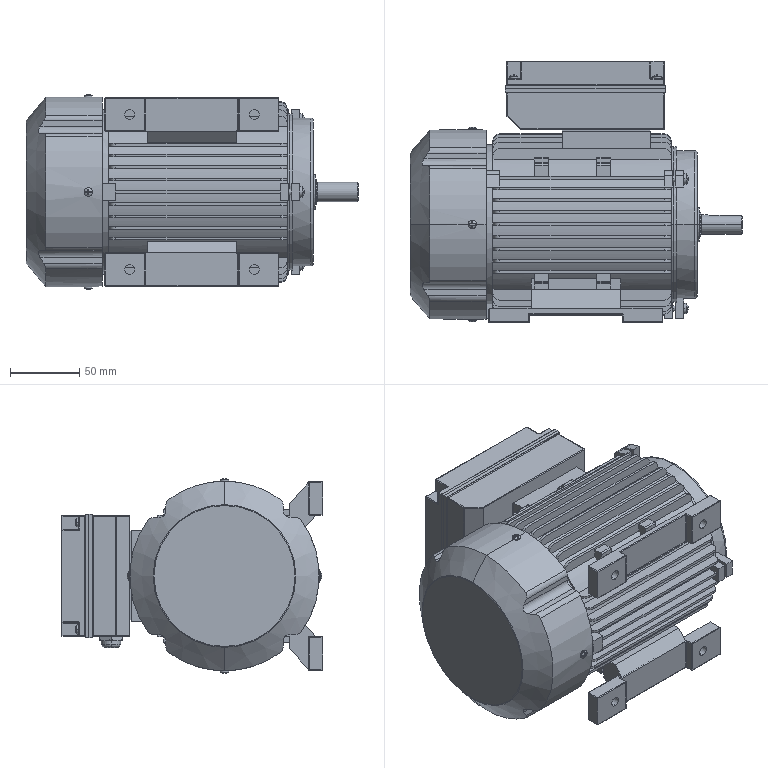Part | SolidWorks | features BaseBody 1 | 1 solid | 1005 faces | box 240 x 189 x 140.895 mm | volume 3047126 mm3 | plane 525 | cylinder 372 | sphere 55 | torus 32 | cone 21 | commonest cylinder face diameters 1 x120 10 x93 117.5 x47 2 x20 6 x16 4 x14